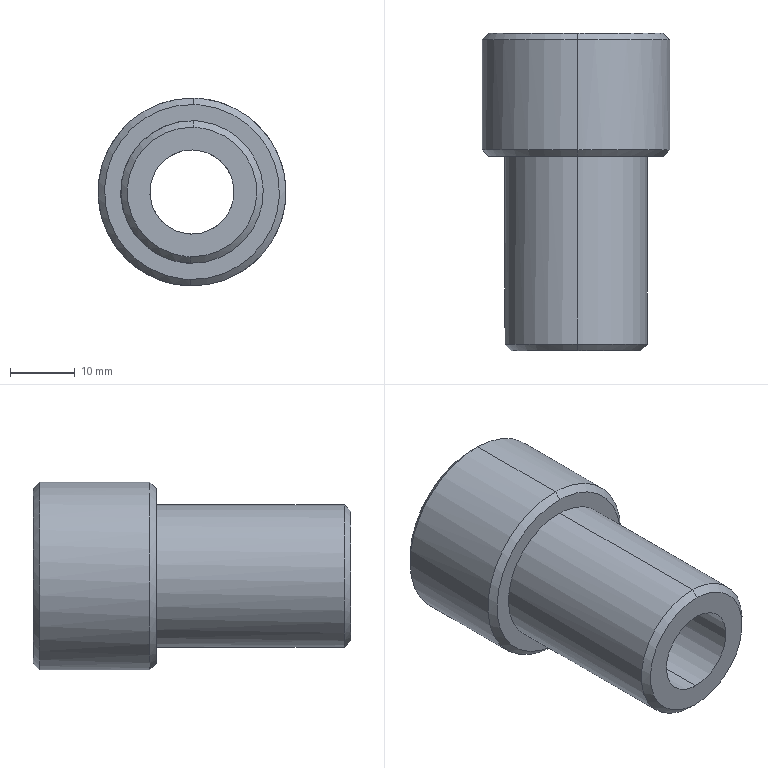Part | Creo | 1 solid | 18 faces | box 29 x 49 x 29 mm | volume 14969 mm3 | cylinder 8 | cone 6 | plane 4 | commonest cylinder face diameters 13 x2 20 x2 22 x2 29 x2
STEP:
#1=CARTESIAN_POINT('',(65.53,388.,-134.74));
#2=VERTEX_POINT('',#1);
#3=CARTESIAN_POINT('',(67.299,388.,-105.822));
#4=VERTEX_POINT('',#3);
#5=CARTESIAN_POINT('',(67.046,388.,-120.32));
#6=DIRECTION('',(0.,1.,0.));
#7=DIRECTION('',(-0.1045,0.,-0.9945));
#8=AXIS2_PLACEMENT_3D('',#5,#6,#7);
#9=CIRCLE('',#8,14.5);
#10=EDGE_CURVE('',#2,#4,#9,.T.);
#11=ORIENTED_EDGE('',*,*,#10,.F.);
#12=CARTESIAN_POINT('',(66.793,388.,-134.817));
#13=VERTEX_POINT('',#12);
#14=CARTESIAN_POINT('',(67.046,388.,-120.32));
#15=DIRECTION('',(0.,1.,0.));
#16=DIRECTION('',(-0.01745,0.,-0.9998));
#17=AXIS2_PLACEMENT_3D('',#14,#15,#16);
#18=CIRCLE('',#17,14.5);
#19=EDGE_CURVE('',#13,#2,#18,.T.);
#20=ORIENTED_EDGE('',*,*,#19,.F.);
#21=CARTESIAN_POINT('',(66.81,389.,-133.818));
#22=VERTEX_POINT('',#21);
#23=CARTESIAN_POINT('',(66.81,389.,-133.818));
#24=DIRECTION('',(-0.01234,-0.7071,-0.707));
#25=VECTOR('',#24,1.414);
#26=LINE('',#23,#25);
#27=EDGE_CURVE('',#22,#13,#26,.T.);
#28=ORIENTED_EDGE('',*,*,#27,.F.);
#29=CARTESIAN_POINT('',(65.635,389.,-133.746));
#30=VERTEX_POINT('',#29);
#31=CARTESIAN_POINT('',(67.046,389.,-120.32));
#32=DIRECTION('',(0.,1.,0.));
#33=DIRECTION('',(-0.01745,0.,-0.9998));
#34=AXIS2_PLACEMENT_3D('',#31,#32,#33);
#35=CIRCLE('',#34,13.5);
#36=EDGE_CURVE('',#22,#30,#35,.T.);
#37=ORIENTED_EDGE('',*,*,#36,.T.);
#38=CARTESIAN_POINT('',(67.281,389.,-106.822));
#39=VERTEX_POINT('',#38);
#40=CARTESIAN_POINT('',(67.046,389.,-120.32));
#41=DIRECTION('',(0.,1.,0.));
#42=DIRECTION('',(-0.1045,0.,-0.9945));
#43=AXIS2_PLACEMENT_3D('',#40,#41,#42);
#44=CIRCLE('',#43,13.5);
#45=EDGE_CURVE('',#30,#39,#44,.T.);
#46=ORIENTED_EDGE('',*,*,#45,.T.);
#47=CARTESIAN_POINT('',(67.281,389.,-106.822));
#48=DIRECTION('',(0.01234,-0.7071,0.707));
#49=VECTOR('',#48,1.414);
#50=LINE('',#47,#49);
#51=EDGE_CURVE('',#39,#4,#50,.T.);
#52=ORIENTED_EDGE('',*,*,#51,.T.);
#53=EDGE_LOOP('',(#11,#20,#28,#37,#46,#52));
#54=FACE_OUTER_BOUND('',#53,.F.);
#55=CARTESIAN_POINT('',(67.046,388.5,-120.32));
#56=DIRECTION('',(0.,-1.,0.));
#57=DIRECTION('',(0.01745,0.,0.9998));
#58=AXIS2_PLACEMENT_3D('',#55,#56,#57);
#59=CONICAL_SURFACE('',#58,14.,45.);
#60=ADVANCED_FACE('',(#54),#59,.T.);
#61=ORIENTED_EDGE('',*,*,#19,.T.);
#62=ORIENTED_EDGE('',*,*,#10,.T.);
#63=CARTESIAN_POINT('',(67.299,371.,-105.822));
#64=VERTEX_POINT('',#63);
#65=CARTESIAN_POINT('',(67.299,371.,-105.822));
#66=DIRECTION('',(0.,1.,0.));
#67=VECTOR('',#66,17.);
#68=LINE('',#65,#67);
#69=EDGE_CURVE('',#64,#4,#68,.T.);
#70=ORIENTED_EDGE('',*,*,#69,.F.);
#71=CARTESIAN_POINT('',(66.793,371.,-134.817));
#72=VERTEX_POINT('',#71);
#73=CARTESIAN_POINT('',(67.046,371.,-120.32));
#74=DIRECTION('',(0.,-1.,0.));
#75=DIRECTION('',(0.01745,0.,0.9998));
#76=AXIS2_PLACEMENT_3D('',#73,#74,#75);
#77=CIRCLE('',#76,14.5);
#78=EDGE_CURVE('',#64,#72,#77,.T.);
#79=ORIENTED_EDGE('',*,*,#78,.T.);
#80=CARTESIAN_POINT('',(66.793,371.,-134.817));
#81=DIRECTION('',(0.,1.,0.));
#82=VECTOR('',#81,17.);
#83=LINE('',#80,#82);
#84=EDGE_CURVE('',#72,#13,#83,.T.);
#85=ORIENTED_EDGE('',*,*,#84,.T.);
#86=EDGE_LOOP('',(#61,#62,#70,#79,#85));
#87=FACE_OUTER_BOUND('',#86,.F.);
#88=CARTESIAN_POINT('',(67.046,370.,-120.32));
#89=DIRECTION('',(0.,1.,0.));
#90=DIRECTION('',(-0.01745,0.,-0.9998));
#91=AXIS2_PLACEMENT_3D('',#88,#89,#90);
#92=CYLINDRICAL_SURFACE('',#91,14.5);
#93=ADVANCED_FACE('',(#87),#92,.T.);
#94=CARTESIAN_POINT('',(67.046,388.,-120.32));
#95=DIRECTION('',(0.,1.,0.));
#96=DIRECTION('',(0.01745,0.,0.9998));
#97=AXIS2_PLACEMENT_3D('',#94,#95,#96);
#98=CIRCLE('',#97,14.5);
#99=EDGE_CURVE('',#4,#13,#98,.T.);
#100=ORIENTED_EDGE('',*,*,#99,.T.);
#101=ORIENTED_EDGE('',*,*,#84,.F.);
#102=CARTESIAN_POINT('',(68.561,371.,-105.899));
#103=VERTEX_POINT('',#102);
#104=CARTESIAN_POINT('',(67.046,371.,-120.32));
#105=DIRECTION('',(0.,-1.,0.));
#106=DIRECTION('',(-0.01745,0.,-0.9998));
#107=AXIS2_PLACEMENT_3D('',#104,#105,#106);
#108=CIRCLE('',#107,14.5);
#109=EDGE_CURVE('',#72,#103,#108,.T.);
#110=ORIENTED_EDGE('',*,*,#109,.T.);
#111=CARTESIAN_POINT('',(67.046,371.,-120.32));
#112=DIRECTION('',(0.,-1.,0.));
#113=DIRECTION('',(0.1045,0.,0.9945));
#114=AXIS2_PLACEMENT_3D('',#111,#112,#113);
#115=CIRCLE('',#114,14.5);
#116=EDGE_CURVE('',#103,#64,#115,.T.);
#117=ORIENTED_EDGE('',*,*,#116,.T.);
#118=ORIENTED_EDGE('',*,*,#69,.T.);
#119=EDGE_LOOP('',(#100,#101,#110,#117,#118));
#120=FACE_OUTER_BOUND('',#119,.F.);
#121=CARTESIAN_POINT('',(67.046,370.,-120.32));
#122=DIRECTION('',(0.,1.,0.));
#123=DIRECTION('',(-0.01745,0.,-0.9998));
#124=AXIS2_PLACEMENT_3D('',#121,#122,#123);
#125=CYLINDRICAL_SURFACE('',#124,14.5);
#126=ADVANCED_FACE('',(#120),#125,.T.);
#127=ORIENTED_EDGE('',*,*,#99,.F.);
#128=ORIENTED_EDGE('',*,*,#51,.F.);
#129=CARTESIAN_POINT('',(68.457,389.,-106.894));
#130=VERTEX_POINT('',#129);
#131=CARTESIAN_POINT('',(67.046,389.,-120.32));
#132=DIRECTION('',(0.,1.,0.));
#133=DIRECTION('',(0.01745,0.,0.9998));
#134=AXIS2_PLACEMENT_3D('',#131,#132,#133);
#135=CIRCLE('',#134,13.5);
#136=EDGE_CURVE('',#39,#130,#135,.T.);
#137=ORIENTED_EDGE('',*,*,#136,.T.);
#138=CARTESIAN_POINT('',(67.046,389.,-120.32));
#139=DIRECTION('',(0.,1.,0.));
#140=DIRECTION('',(0.1045,0.,0.9945));
#141=AXIS2_PLACEMENT_3D('',#138,#139,#140);
#142=CIRCLE('',#141,13.5);
#143=EDGE_CURVE('',#130,#22,#142,.T.);
#144=ORIENTED_EDGE('',*,*,#143,.T.);
#145=ORIENTED_EDGE('',*,*,#27,.T.);
#146=EDGE_LOOP('',(#127,#128,#137,#144,#145));
#147=FACE_OUTER_BOUND('',#146,.F.);
#148=CARTESIAN_POINT('',(67.046,388.5,-120.32));
#149=DIRECTION('',(0.,-1.,0.));
#150=DIRECTION('',(0.01745,0.,0.9998));
#151=AXIS2_PLACEMENT_3D('',#148,#149,#150);
#152=CONICAL_SURFACE('',#151,14.,45.);
#153=ADVANCED_FACE('',(#147),#152,.T.);
#154=ORIENTED_EDGE('',*,*,#45,.F.);
#155=ORIENTED_EDGE('',*,*,#36,.F.);
#156=ORIENTED_EDGE('',*,*,#143,.F.);
#157=ORIENTED_EDGE('',*,*,#136,.F.);
#158=EDGE_LOOP('',(#154,#155,#156,#157));
#159=FACE_OUTER_BOUND('',#158,.F.);
#160=CARTESIAN_POINT('',(66.001,389.,-130.265));
#161=VERTEX_POINT('',#160);
#162=CARTESIAN_POINT('',(66.871,389.,-130.318));
#163=VERTEX_POINT('',#162);
#164=CARTESIAN_POINT('',(67.046,389.,-120.32));
#165=DIRECTION('',(0.,-1.,0.));
#166=DIRECTION('',(-0.1045,0.,-0.9945));
#167=AXIS2_PLACEMENT_3D('',#164,#165,#166);
#168=CIRCLE('',#167,10.);
#169=EDGE_CURVE('',#161,#163,#168,.T.);
#170=ORIENTED_EDGE('',*,*,#169,.F.);
#171=CARTESIAN_POINT('',(67.22,389.,-110.321));
#172=VERTEX_POINT('',#171);
#173=CARTESIAN_POINT('',(67.046,389.,-120.32));
#174=DIRECTION('',(0.,-1.,0.));
#175=DIRECTION('',(0.01745,0.,0.9998));
#176=AXIS2_PLACEMENT_3D('',#173,#174,#175);
#177=CIRCLE('',#176,10.);
#178=EDGE_CURVE('',#172,#161,#177,.T.);
#179=ORIENTED_EDGE('',*,*,#178,.F.);
#180=CARTESIAN_POINT('',(67.046,389.,-120.32));
#181=DIRECTION('',(0.,-1.,0.));
#182=DIRECTION('',(-0.01745,0.,-0.9998));
#183=AXIS2_PLACEMENT_3D('',#180,#181,#182);
#184=CIRCLE('',#183,10.);
#185=EDGE_CURVE('',#163,#172,#184,.T.);
#186=ORIENTED_EDGE('',*,*,#185,.F.);
#187=EDGE_LOOP('',(#170,#179,#186));
#188=FACE_BOUND('',#187,.F.);
#189=CARTESIAN_POINT('',(13.059,389.,16.573));
#190=DIRECTION('',(0.,1.,0.));
#191=DIRECTION('',(-0.01745,0.,-0.9998));
#192=AXIS2_PLACEMENT_3D('',#189,#190,#191);
#193=PLANE('',#192);
#194=ADVANCED_FACE('',(#159,#188),#193,.T.);
#195=CARTESIAN_POINT('',(66.871,376.,-130.318));
#196=VERTEX_POINT('',#195);
#197=CARTESIAN_POINT('',(66.348,376.,-110.344));
#198=VERTEX_POINT('',#197);
#199=CARTESIAN_POINT('',(67.046,376.,-120.32));
#200=DIRECTION('',(0.,1.,0.));
#201=DIRECTION('',(-0.01745,0.,-0.9998));
#202=AXIS2_PLACEMENT_3D('',#199,#200,#201);
#203=CIRCLE('',#202,10.);
#204=EDGE_CURVE('',#196,#198,#203,.T.);
#205=ORIENTED_EDGE('',*,*,#204,.T.);
#206=CARTESIAN_POINT('',(67.22,376.,-110.321));
#207=VERTEX_POINT('',#206);
#208=CARTESIAN_POINT('',(67.046,376.,-120.32));
#209=DIRECTION('',(0.,1.,0.));
#210=DIRECTION('',(-0.06976,0.,0.9976));
#211=AXIS2_PLACEMENT_3D('',#208,#209,#210);
#212=CIRCLE('',#211,10.);
#213=EDGE_CURVE('',#198,#207,#212,.T.);
#214=ORIENTED_EDGE('',*,*,#213,.T.);
#215=CARTESIAN_POINT('',(67.22,376.,-110.321));
#216=DIRECTION('',(0.,1.,0.));
#217=VECTOR('',#216,13.);
#218=LINE('',#215,#217);
#219=EDGE_CURVE('',#207,#172,#218,.T.);
#220=ORIENTED_EDGE('',*,*,#219,.T.);
#221=ORIENTED_EDGE('',*,*,#178,.T.);
#222=ORIENTED_EDGE('',*,*,#169,.T.);
#223=CARTESIAN_POINT('',(66.871,376.,-130.318));
#224=DIRECTION('',(0.,1.,0.));
#225=VECTOR('',#224,13.);
#226=LINE('',#223,#225);
#227=EDGE_CURVE('',#196,#163,#226,.T.);
#228=ORIENTED_EDGE('',*,*,#227,.F.);
#229=EDGE_LOOP('',(#205,#214,#220,#221,#222,#228));
#230=FACE_OUTER_BOUND('',#229,.F.);
#231=CARTESIAN_POINT('',(67.046,389.,-120.32));
#232=DIRECTION('',(0.,1.,0.));
#233=DIRECTION('',(-0.01745,0.,-0.9998));
#234=AXIS2_PLACEMENT_3D('',#231,#232,#233);
#235=CYLINDRICAL_SURFACE('',#234,10.);
#236=ADVANCED_FACE('',(#230),#235,.F.);
#237=ORIENTED_EDGE('',*,*,#213,.F.);
#238=ORIENTED_EDGE('',*,*,#204,.F.);
#239=CARTESIAN_POINT('',(67.743,376.,-130.295));
#240=VERTEX_POINT('',#239);
#241=CARTESIAN_POINT('',(67.046,376.,-120.32));
#242=DIRECTION('',(0.,1.,0.));
#243=DIRECTION('',(0.06976,0.,-0.9976));
#244=AXIS2_PLACEMENT_3D('',#241,#242,#243);
#245=CIRCLE('',#244,10.);
#246=EDGE_CURVE('',#240,#196,#245,.T.);
#247=ORIENTED_EDGE('',*,*,#246,.F.);
#248=CARTESIAN_POINT('',(67.046,376.,-120.32));
#249=DIRECTION('',(0.,1.,0.));
#250=DIRECTION('',(0.01745,0.,0.9998));
#251=AXIS2_PLACEMENT_3D('',#248,#249,#250);
#252=CIRCLE('',#251,10.);
#253=EDGE_CURVE('',#207,#240,#252,.T.);
#254=ORIENTED_EDGE('',*,*,#253,.F.);
#255=EDGE_LOOP('',(#237,#238,#247,#254));
#256=FACE_OUTER_BOUND('',#255,.F.);
#257=CARTESIAN_POINT('',(67.725,376.,-113.855));
#258=VERTEX_POINT('',#257);
#259=CARTESIAN_POINT('',(67.159,376.,-113.821));
#260=VERTEX_POINT('',#259);
#261=CARTESIAN_POINT('',(67.046,376.,-120.32));
#262=DIRECTION('',(0.,-1.,0.));
#263=DIRECTION('',(0.1045,0.,0.9945));
#264=AXIS2_PLACEMENT_3D('',#261,#262,#263);
#265=CIRCLE('',#264,6.5);
#266=EDGE_CURVE('',#258,#260,#265,.T.);
#267=ORIENTED_EDGE('',*,*,#266,.F.);
#268=CARTESIAN_POINT('',(66.932,376.,-126.819));
#269=VERTEX_POINT('',#268);
#270=CARTESIAN_POINT('',(67.046,376.,-120.32));
#271=DIRECTION('',(0.,-1.,0.));
#272=DIRECTION('',(-0.01745,0.,-0.9998));
#273=AXIS2_PLACEMENT_3D('',#270,#271,#272);
#274=CIRCLE('',#273,6.5);
#275=EDGE_CURVE('',#269,#258,#274,.T.);
#276=ORIENTED_EDGE('',*,*,#275,.F.);
#277=CARTESIAN_POINT('',(67.046,376.,-120.32));
#278=DIRECTION('',(0.,-1.,0.));
#279=DIRECTION('',(0.01745,0.,0.9998));
#280=AXIS2_PLACEMENT_3D('',#277,#278,#279);
#281=CIRCLE('',#280,6.5);
#282=EDGE_CURVE('',#260,#269,#281,.T.);
#283=ORIENTED_EDGE('',*,*,#282,.F.);
#284=EDGE_LOOP('',(#267,#276,#283));
#285=FACE_BOUND('',#284,.F.);
#286=CARTESIAN_POINT('',(67.046,376.,-120.32));
#287=DIRECTION('',(0.,-1.,0.));
#288=DIRECTION('',(0.01745,0.,0.9998));
#289=AXIS2_PLACEMENT_3D('',#286,#287,#288);
#290=PLANE('',#289);
#291=ADVANCED_FACE('',(#256,#285),#290,.F.);
#292=ORIENTED_EDGE('',*,*,#246,.T.);
#293=ORIENTED_EDGE('',*,*,#227,.T.);
#294=ORIENTED_EDGE('',*,*,#185,.T.);
#295=ORIENTED_EDGE('',*,*,#219,.F.);
#296=ORIENTED_EDGE('',*,*,#253,.T.);
#297=EDGE_LOOP('',(#292,#293,#294,#295,#296));
#298=FACE_OUTER_BOUND('',#297,.F.);
#299=CARTESIAN_POINT('',(67.046,389.,-120.32));
#300=DIRECTION('',(0.,1.,0.));
#301=DIRECTION('',(-0.01745,0.,-0.9998));
#302=AXIS2_PLACEMENT_3D('',#299,#300,#301);
#303=CYLINDRICAL_SURFACE('',#302,10.);
#304=ADVANCED_FACE('',(#298),#303,.F.);
#305=ORIENTED_EDGE('',*,*,#275,.T.);
#306=ORIENTED_EDGE('',*,*,#266,.T.);
#307=CARTESIAN_POINT('',(67.159,340.,-113.821));
#308=VERTEX_POINT('',#307);
#309=CARTESIAN_POINT('',(67.159,340.,-113.821));
#310=DIRECTION('',(0.,1.,0.));
#311=VECTOR('',#310,36.);
#312=LINE('',#309,#311);
#313=EDGE_CURVE('',#308,#260,#312,.T.);
#314=ORIENTED_EDGE('',*,*,#313,.F.);
#315=CARTESIAN_POINT('',(66.932,340.,-126.819));
#316=VERTEX_POINT('',#315);
#317=CARTESIAN_POINT('',(67.046,340.,-120.32));
#318=DIRECTION('',(0.,1.,0.));
#319=DIRECTION('',(0.01745,0.,0.9998));
#320=AXIS2_PLACEMENT_3D('',#317,#318,#319);
#321=CIRCLE('',#320,6.5);
#322=EDGE_CURVE('',#308,#316,#321,.T.);
#323=ORIENTED_EDGE('',*,*,#322,.T.);
#324=CARTESIAN_POINT('',(66.932,340.,-126.819));
#325=DIRECTION('',(0.,1.,0.));
#326=VECTOR('',#325,36.);
#327=LINE('',#324,#326);
#328=EDGE_CURVE('',#316,#269,#327,.T.);
#329=ORIENTED_EDGE('',*,*,#328,.T.);
#330=EDGE_LOOP('',(#305,#306,#314,#323,#329));
#331=FACE_OUTER_BOUND('',#330,.F.);
#332=CARTESIAN_POINT('',(67.046,340.,-120.32));
#333=DIRECTION('',(0.,1.,0.));
#334=DIRECTION('',(-0.01745,0.,-0.9998));
#335=AXIS2_PLACEMENT_3D('',#332,#333,#334);
#336=CYLINDRICAL_SURFACE('',#335,6.5);
#337=ADVANCED_FACE('',(#331),#336,.F.);
#338=ORIENTED_EDGE('',*,*,#282,.T.);
#339=ORIENTED_EDGE('',*,*,#328,.F.);
#340=CARTESIAN_POINT('',(66.366,340.,-126.784));
#341=VERTEX_POINT('',#340);
#342=CARTESIAN_POINT('',(67.046,340.,-120.32));
#343=DIRECTION('',(0.,1.,0.));
#344=DIRECTION('',(-0.01745,0.,-0.9998));
#345=AXIS2_PLACEMENT_3D('',#342,#343,#344);
#346=CIRCLE('',#345,6.5);
#347=EDGE_CURVE('',#316,#341,#346,.T.);
#348=ORIENTED_EDGE('',*,*,#347,.T.);
#349=CARTESIAN_POINT('',(67.046,340.,-120.32));
#350=DIRECTION('',(0.,1.,0.));
#351=DIRECTION('',(-0.1045,0.,-0.9945));
#352=AXIS2_PLACEMENT_3D('',#349,#350,#351);
#353=CIRCLE('',#352,6.5);
#354=EDGE_CURVE('',#341,#308,#353,.T.);
#355=ORIENTED_EDGE('',*,*,#354,.T.);
#356=ORIENTED_EDGE('',*,*,#313,.T.);
#357=EDGE_LOOP('',(#338,#339,#348,#355,#356));
#358=FACE_OUTER_BOUND('',#357,.F.);
#359=CARTESIAN_POINT('',(67.046,340.,-120.32));
#360=DIRECTION('',(0.,1.,0.));
#361=DIRECTION('',(-0.01745,0.,-0.9998));
#362=AXIS2_PLACEMENT_3D('',#359,#360,#361);
#363=CYLINDRICAL_SURFACE('',#362,6.5);
#364=ADVANCED_FACE('',(#358),#363,.F.);
#365=CARTESIAN_POINT('',(68.091,340.,-110.374));
#366=VERTEX_POINT('',#365);
#367=CARTESIAN_POINT('',(67.22,340.,-110.321));
#368=VERTEX_POINT('',#367);
#369=CARTESIAN_POINT('',(67.046,340.,-120.32));
#370=DIRECTION('',(0.,-1.,0.));
#371=DIRECTION('',(0.1045,0.,0.9945));
#372=AXIS2_PLACEMENT_3D('',#369,#370,#371);
#373=CIRCLE('',#372,10.);
#374=EDGE_CURVE('',#366,#368,#373,.T.);
#375=ORIENTED_EDGE('',*,*,#374,.F.);
#376=CARTESIAN_POINT('',(66.871,340.,-130.318));
#377=VERTEX_POINT('',#376);
#378=CARTESIAN_POINT('',(67.046,340.,-120.32));
#379=DIRECTION('',(0.,-1.,0.));
#380=DIRECTION('',(-0.01745,0.,-0.9998));
#381=AXIS2_PLACEMENT_3D('',#378,#379,#380);
#382=CIRCLE('',#381,10.);
#383=EDGE_CURVE('',#377,#366,#382,.T.);
#384=ORIENTED_EDGE('',*,*,#383,.F.);
#385=CARTESIAN_POINT('',(66.001,340.,-130.265));
#386=VERTEX_POINT('',#385);
#387=CARTESIAN_POINT('',(67.046,340.,-120.32));
#388=DIRECTION('',(0.,-1.,0.));
#389=DIRECTION('',(-0.1045,0.,-0.9945));
#390=AXIS2_PLACEMENT_3D('',#387,#388,#389);
#391=CIRCLE('',#390,10.);
#392=EDGE_CURVE('',#386,#377,#391,.T.);
#393=ORIENTED_EDGE('',*,*,#392,.F.);
#394=CARTESIAN_POINT('',(67.046,340.,-120.32));
#395=DIRECTION('',(0.,-1.,0.));
#396=DIRECTION('',(0.01745,0.,0.9998));
#397=AXIS2_PLACEMENT_3D('',#394,#395,#396);
#398=CIRCLE('',#397,10.);
#399=EDGE_CURVE('',#368,#386,#398,.T.);
#400=ORIENTED_EDGE('',*,*,#399,.F.);
#401=EDGE_LOOP('',(#375,#384,#393,#400));
#402=FACE_OUTER_BOUND('',#401,.F.);
#403=ORIENTED_EDGE('',*,*,#354,.F.);
#404=ORIENTED_EDGE('',*,*,#347,.F.);
#405=ORIENTED_EDGE('',*,*,#322,.F.);
#406=EDGE_LOOP('',(#403,#404,#405));
#407=FACE_BOUND('',#406,.F.);
#408=CARTESIAN_POINT('',(13.059,340.,16.573));
#409=DIRECTION('',(0.,1.,0.));
#410=DIRECTION('',(-0.01745,0.,-0.9998));
#411=AXIS2_PLACEMENT_3D('',#408,#409,#410);
#412=PLANE('',#411);
#413=ADVANCED_FACE('',(#402,#407),#412,.F.);
#414=CARTESIAN_POINT('',(68.196,341.,-109.38));
#415=VERTEX_POINT('',#414);
#416=CARTESIAN_POINT('',(67.238,341.,-109.321));
#417=VERTEX_POINT('',#416);
#418=CARTESIAN_POINT('',(67.046,341.,-120.32));
#419=DIRECTION('',(0.,-1.,0.));
#420=DIRECTION('',(0.1045,0.,0.9945));
#421=AXIS2_PLACEMENT_3D('',#418,#419,#420);
#422=CIRCLE('',#421,11.);
#423=EDGE_CURVE('',#415,#417,#422,.T.);
#424=ORIENTED_EDGE('',*,*,#423,.F.);
#425=CARTESIAN_POINT('',(66.854,341.,-131.318));
#426=VERTEX_POINT('',#425);
#427=CARTESIAN_POINT('',(67.046,341.,-120.32));
#428=DIRECTION('',(0.,-1.,0.));
#429=DIRECTION('',(-0.01745,0.,-0.9998));
#430=AXIS2_PLACEMENT_3D('',#427,#428,#429);
#431=CIRCLE('',#430,11.);
#432=EDGE_CURVE('',#426,#415,#431,.T.);
#433=ORIENTED_EDGE('',*,*,#432,.F.);
#434=CARTESIAN_POINT('',(66.871,340.,-130.318));
#435=DIRECTION('',(-0.01234,0.7071,-0.707));
#436=VECTOR('',#435,1.414);
#437=LINE('',#434,#436);
#438=EDGE_CURVE('',#377,#426,#437,.T.);
#439=ORIENTED_EDGE('',*,*,#438,.F.);
#440=ORIENTED_EDGE('',*,*,#383,.T.);
#441=ORIENTED_EDGE('',*,*,#374,.T.);
#442=CARTESIAN_POINT('',(67.22,340.,-110.321));
#443=DIRECTION('',(0.01234,0.7071,0.707));
#444=VECTOR('',#443,1.414);
#445=LINE('',#442,#444);
#446=EDGE_CURVE('',#368,#417,#445,.T.);
#447=ORIENTED_EDGE('',*,*,#446,.T.);
#448=EDGE_LOOP('',(#424,#433,#439,#440,#441,#447));
#449=FACE_OUTER_BOUND('',#448,.F.);
#450=CARTESIAN_POINT('',(67.046,340.5,-120.32));
#451=DIRECTION('',(0.,1.,0.));
#452=DIRECTION('',(-0.01745,0.,-0.9998));
#453=AXIS2_PLACEMENT_3D('',#450,#451,#452);
#454=CONICAL_SURFACE('',#453,10.5,45.);
#455=ADVANCED_FACE('',(#449),#454,.T.);
#456=CARTESIAN_POINT('',(67.238,370.,-109.321));
#457=VERTEX_POINT('',#456);
#458=CARTESIAN_POINT('',(68.196,370.,-109.38));
#459=VERTEX_POINT('',#458);
#460=CARTESIAN_POINT('',(67.046,370.,-120.32));
#461=DIRECTION('',(0.,1.,0.));
#462=DIRECTION('',(0.01745,0.,0.9998));
#463=AXIS2_PLACEMENT_3D('',#460,#461,#462);
#464=CIRCLE('',#463,11.);
#465=EDGE_CURVE('',#457,#459,#464,.T.);
#466=ORIENTED_EDGE('',*,*,#465,.T.);
#467=CARTESIAN_POINT('',(66.854,370.,-131.318));
#468=VERTEX_POINT('',#467);
#469=CARTESIAN_POINT('',(67.046,370.,-120.32));
#470=DIRECTION('',(0.,1.,0.));
#471=DIRECTION('',(0.1045,0.,0.9945));
#472=AXIS2_PLACEMENT_3D('',#469,#470,#471);
#473=CIRCLE('',#472,11.);
#474=EDGE_CURVE('',#459,#468,#473,.T.);
#475=ORIENTED_EDGE('',*,*,#474,.T.);
#476=CARTESIAN_POINT('',(66.854,341.,-131.318));
#477=DIRECTION('',(0.,1.,0.));
#478=VECTOR('',#477,29.);
#479=LINE('',#476,#478);
#480=EDGE_CURVE('',#426,#468,#479,.T.);
#481=ORIENTED_EDGE('',*,*,#480,.F.);
#482=ORIENTED_EDGE('',*,*,#432,.T.);
#483=ORIENTED_EDGE('',*,*,#423,.T.);
#484=CARTESIAN_POINT('',(67.238,341.,-109.321));
#485=DIRECTION('',(0.,1.,0.));
#486=VECTOR('',#485,29.);
#487=LINE('',#484,#486);
#488=EDGE_CURVE('',#417,#457,#487,.T.);
#489=ORIENTED_EDGE('',*,*,#488,.T.);
#490=EDGE_LOOP('',(#466,#475,#481,#482,#483,#489));
#491=FACE_OUTER_BOUND('',#490,.F.);
#492=CARTESIAN_POINT('',(67.046,340.,-120.32));
#493=DIRECTION('',(0.,1.,0.));
#494=DIRECTION('',(-0.01745,0.,-0.9998));
#495=AXIS2_PLACEMENT_3D('',#492,#493,#494);
#496=CYLINDRICAL_SURFACE('',#495,11.);
#497=ADVANCED_FACE('',(#491),#496,.T.);
#498=CARTESIAN_POINT('',(68.457,370.,-106.894));
#499=VERTEX_POINT('',#498);
#500=CARTESIAN_POINT('',(67.281,370.,-106.822));
#501=VERTEX_POINT('',#500);
#502=CARTESIAN_POINT('',(67.046,370.,-120.32));
#503=DIRECTION('',(0.,-1.,0.));
#504=DIRECTION('',(0.1045,0.,0.9945));
#505=AXIS2_PLACEMENT_3D('',#502,#503,#504);
#506=CIRCLE('',#505,13.5);
#507=EDGE_CURVE('',#499,#501,#506,.T.);
#508=ORIENTED_EDGE('',*,*,#507,.F.);
#509=CARTESIAN_POINT('',(66.81,370.,-133.818));
#510=VERTEX_POINT('',#509);
#511=CARTESIAN_POINT('',(67.046,370.,-120.32));
#512=DIRECTION('',(0.,-1.,0.));
#513=DIRECTION('',(-0.01745,0.,-0.9998));
#514=AXIS2_PLACEMENT_3D('',#511,#512,#513);
#515=CIRCLE('',#514,13.5);
#516=EDGE_CURVE('',#510,#499,#515,.T.);
#517=ORIENTED_EDGE('',*,*,#516,.F.);
#518=CARTESIAN_POINT('',(65.635,370.,-133.746));
#519=VERTEX_POINT('',#518);
#520=CARTESIAN_POINT('',(67.046,370.,-120.32));
#521=DIRECTION('',(0.,-1.,0.));
#522=DIRECTION('',(-0.1045,0.,-0.9945));
#523=AXIS2_PLACEMENT_3D('',#520,#521,#522);
#524=CIRCLE('',#523,13.5);
#525=EDGE_CURVE('',#519,#510,#524,.T.);
#526=ORIENTED_EDGE('',*,*,#525,.F.);
#527=CARTESIAN_POINT('',(67.046,370.,-120.32));
#528=DIRECTION('',(0.,-1.,0.));
#529=DIRECTION('',(0.01745,0.,0.9998));
#530=AXIS2_PLACEMENT_3D('',#527,#528,#529);
#531=CIRCLE('',#530,13.5);
#532=EDGE_CURVE('',#501,#519,#531,.T.);
#533=ORIENTED_EDGE('',*,*,#532,.F.);
#534=EDGE_LOOP('',(#508,#517,#526,#533));
#535=FACE_OUTER_BOUND('',#534,.F.);
#536=ORIENTED_EDGE('',*,*,#474,.F.);
#537=ORIENTED_EDGE('',*,*,#465,.F.);
#538=CARTESIAN_POINT('',(65.896,370.,-131.259));
#539=VERTEX_POINT('',#538);
#540=CARTESIAN_POINT('',(67.046,370.,-120.32));
#541=DIRECTION('',(0.,1.,0.));
#542=DIRECTION('',(-0.1045,0.,-0.9945));
#543=AXIS2_PLACEMENT_3D('',#540,#541,#542);
#544=CIRCLE('',#543,11.);
#545=EDGE_CURVE('',#539,#457,#544,.T.);
#546=ORIENTED_EDGE('',*,*,#545,.F.);
#547=CARTESIAN_POINT('',(67.046,370.,-120.32));
#548=DIRECTION('',(0.,1.,0.));
#549=DIRECTION('',(-0.01745,0.,-0.9998));
#550=AXIS2_PLACEMENT_3D('',#547,#548,#549);
#551=CIRCLE('',#550,11.);
#552=EDGE_CURVE('',#468,#539,#551,.T.);
#553=ORIENTED_EDGE('',*,*,#552,.F.);
#554=EDGE_LOOP('',(#536,#537,#546,#553));
#555=FACE_BOUND('',#554,.F.);
#556=CARTESIAN_POINT('',(13.059,370.,16.573));
#557=DIRECTION('',(0.,1.,0.));
#558=DIRECTION('',(-0.01745,0.,-0.9998));
#559=AXIS2_PLACEMENT_3D('',#556,#557,#558);
#560=PLANE('',#559);
#561=ADVANCED_FACE('',(#535,#555),#560,.F.);
#562=ORIENTED_EDGE('',*,*,#116,.F.);
#563=ORIENTED_EDGE('',*,*,#109,.F.);
#564=CARTESIAN_POINT('',(66.81,370.,-133.818));
#565=DIRECTION('',(-0.01234,0.7071,-0.707));
#566=VECTOR('',#565,1.414);
#567=LINE('',#564,#566);
#568=EDGE_CURVE('',#510,#72,#567,.T.);
#569=ORIENTED_EDGE('',*,*,#568,.F.);
#570=ORIENTED_EDGE('',*,*,#516,.T.);
#571=ORIENTED_EDGE('',*,*,#507,.T.);
#572=CARTESIAN_POINT('',(67.281,370.,-106.822));
#573=DIRECTION('',(0.01234,0.7071,0.707));
#574=VECTOR('',#573,1.414);
#575=LINE('',#572,#574);
#576=EDGE_CURVE('',#501,#64,#575,.T.);
#577=ORIENTED_EDGE('',*,*,#576,.T.);
#578=EDGE_LOOP('',(#562,#563,#569,#570,#571,#577));
#579=FACE_OUTER_BOUND('',#578,.F.);
#580=CARTESIAN_POINT('',(67.046,370.5,-120.32));
#581=DIRECTION('',(0.,1.,0.));
#582=DIRECTION('',(-0.01745,0.,-0.9998));
#583=AXIS2_PLACEMENT_3D('',#580,#581,#582);
#584=CONICAL_SURFACE('',#583,14.,45.);
#585=ADVANCED_FACE('',(#579),#584,.T.);
#586=ORIENTED_EDGE('',*,*,#78,.F.);
#587=ORIENTED_EDGE('',*,*,#576,.F.);
#588=ORIENTED_EDGE('',*,*,#532,.T.);
#589=ORIENTED_EDGE('',*,*,#525,.T.);
#590=ORIENTED_EDGE('',*,*,#568,.T.);
#591=EDGE_LOOP('',(#586,#587,#588,#589,#590));
#592=FACE_OUTER_BOUND('',#591,.F.);
#593=CARTESIAN_POINT('',(67.046,370.5,-120.32));
#594=DIRECTION('',(0.,1.,0.));
#595=DIRECTION('',(-0.01745,0.,-0.9998));
#596=AXIS2_PLACEMENT_3D('',#593,#594,#595);
#597=CONICAL_SURFACE('',#596,14.,45.);
#598=ADVANCED_FACE('',(#592),#597,.T.);
#599=ORIENTED_EDGE('',*,*,#545,.T.);
#600=ORIENTED_EDGE('',*,*,#488,.F.);
#601=CARTESIAN_POINT('',(67.046,341.,-120.32));
#602=DIRECTION('',(0.,-1.,0.));
#603=DIRECTION('',(0.01745,0.,0.9998));
#604=AXIS2_PLACEMENT_3D('',#601,#602,#603);
#605=CIRCLE('',#604,11.);
#606=EDGE_CURVE('',#417,#426,#605,.T.);
#607=ORIENTED_EDGE('',*,*,#606,.T.);
#608=ORIENTED_EDGE('',*,*,#480,.T.);
#609=ORIENTED_EDGE('',*,*,#552,.T.);
#610=EDGE_LOOP('',(#599,#600,#607,#608,#609));
#611=FACE_OUTER_BOUND('',#610,.F.);
#612=CARTESIAN_POINT('',(67.046,340.,-120.32));
#613=DIRECTION('',(0.,1.,0.));
#614=DIRECTION('',(-0.01745,0.,-0.9998));
#615=AXIS2_PLACEMENT_3D('',#612,#613,#614);
#616=CYLINDRICAL_SURFACE('',#615,11.);
#617=ADVANCED_FACE('',(#611),#616,.T.);
#618=ORIENTED_EDGE('',*,*,#606,.F.);
#619=ORIENTED_EDGE('',*,*,#446,.F.);
#620=ORIENTED_EDGE('',*,*,#399,.T.);
#621=ORIENTED_EDGE('',*,*,#392,.T.);
#622=ORIENTED_EDGE('',*,*,#438,.T.);
#623=EDGE_LOOP('',(#618,#619,#620,#621,#622));
#624=FACE_OUTER_BOUND('',#623,.F.);
#625=CARTESIAN_POINT('',(67.046,340.5,-120.32));
#626=DIRECTION('',(0.,1.,0.));
#627=DIRECTION('',(-0.01745,0.,-0.9998));
#628=AXIS2_PLACEMENT_3D('',#625,#626,#627);
#629=CONICAL_SURFACE('',#628,10.5,45.);
#630=ADVANCED_FACE('',(#624),#629,.T.);
#631=CLOSED_SHELL('',(#60,#93,#126,#153,#194,#236,#291,#304,#337,#364,#413,#455,#497,#561,#585,#598,#617,#630));
#632=MANIFOLD_SOLID_BREP('',#631);
#633=(LENGTH_UNIT()NAMED_UNIT(*)SI_UNIT(.MILLI.,.METRE.));
#634=UNCERTAINTY_MEASURE_WITH_UNIT(LENGTH_MEASURE(0.00639),#633,'','');
#635=(NAMED_UNIT(*)PLANE_ANGLE_UNIT()SI_UNIT($,.RADIAN.));
#636=PLANE_ANGLE_MEASURE_WITH_UNIT(PLANE_ANGLE_MEASURE(0.01745),#635);
#637=(CONVERSION_BASED_UNIT('DEGREE',#636)NAMED_UNIT(*)PLANE_ANGLE_UNIT());
#638=(NAMED_UNIT(*)SI_UNIT($,.STERADIAN.)SOLID_ANGLE_UNIT());
#639=(GEOMETRIC_REPRESENTATION_CONTEXT(3)GLOBAL_UNCERTAINTY_ASSIGNED_CONTEXT((#634))GLOBAL_UNIT_ASSIGNED_CONTEXT((#633,#637,#638))REPRESENTATION_CONTEXT('',''));
#640=ADVANCED_BREP_SHAPE_REPRESENTATION('',(#632),#639);